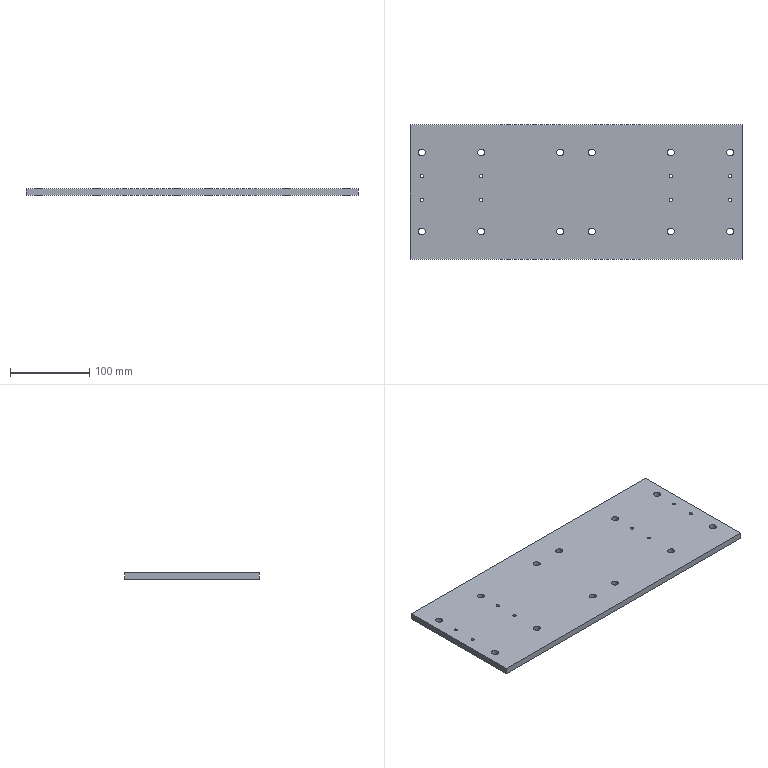Part | 1 solid | 46 faces | box 420 x 170 x 8 mm | volume 564819 mm3 | cylinder 40 | plane 6 | commonest cylinder face diameters 8.6 x24 4 x16